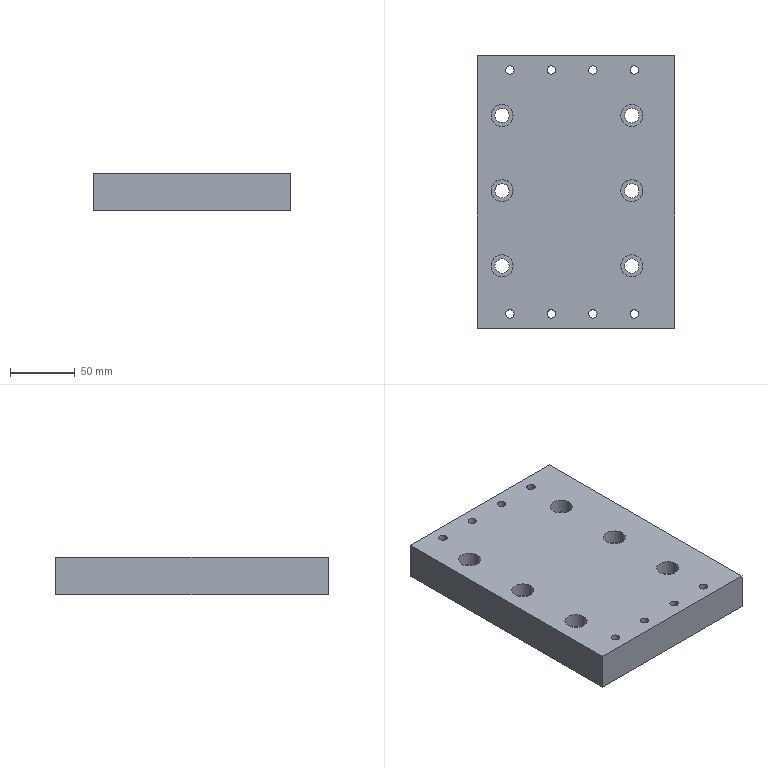Part | STEP file | Turret 32080 Tool Holder Base Plate | 1 solid | 52 faces | box 152 x 210 x 29 mm | volume 892737 mm3 | cylinder 40 | plane 12 | commonest cylinder face diameters 6.5 x16 11 x12 17 x12